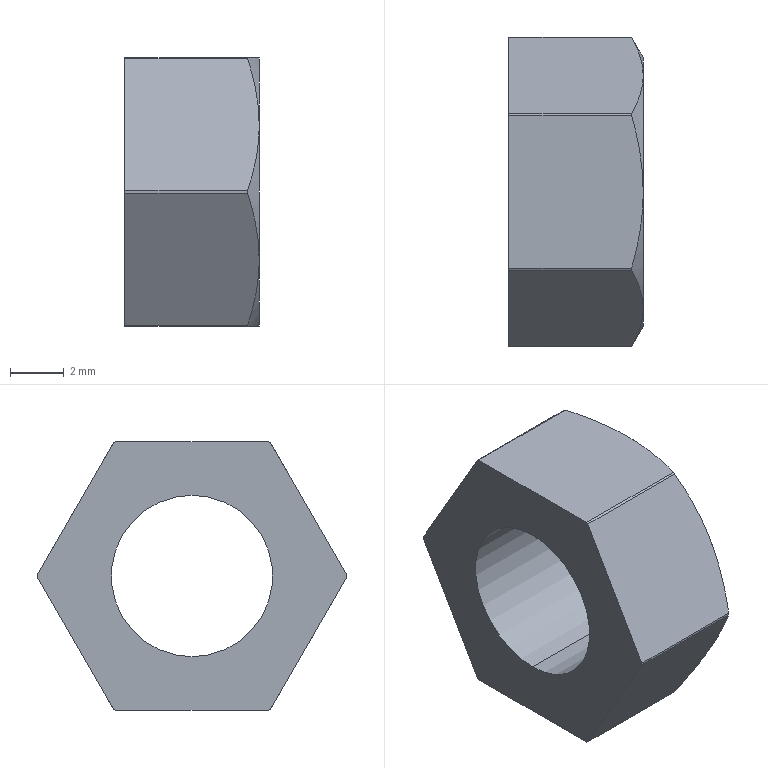Part | STEP file | SSTBB6-25-Part-2-1 | 1 solid | 22 faces | box 5 x 11.5 x 10 mm | volume 290.522 mm3 | cylinder 8 | plane 8 | cone 6 | commonest cylinder face diameters 11.5 x6 6 x2
STEP:
#1=CARTESIAN_POINT('',(12.,0.,3.));
#2=VERTEX_POINT('',#1);
#3=CARTESIAN_POINT('',(12.,0.,-3.));
#4=VERTEX_POINT('',#3);
#5=CARTESIAN_POINT('',(12.,0.,0.));
#6=DIRECTION('',(1.,0.,0.));
#7=DIRECTION('',(0.,0.,1.));
#8=AXIS2_PLACEMENT_3D('',#5,#6,#7);
#9=CIRCLE('',#8,3.);
#10=EDGE_CURVE('',#2,#4,#9,.T.);
#11=ORIENTED_EDGE('',*,*,#10,.T.);
#12=CARTESIAN_POINT('',(7.,0.,-3.));
#13=VERTEX_POINT('',#12);
#14=CARTESIAN_POINT('',(0.,0.,-3.));
#15=DIRECTION('',(-1.,0.,0.));
#16=VECTOR('',#15,1000.);
#17=LINE('',#14,#16);
#18=EDGE_CURVE('',#4,#13,#17,.T.);
#19=ORIENTED_EDGE('',*,*,#18,.T.);
#20=CARTESIAN_POINT('',(7.,0.,3.));
#21=VERTEX_POINT('',#20);
#22=CARTESIAN_POINT('',(7.,0.,0.));
#23=DIRECTION('',(-1.,0.,0.));
#24=DIRECTION('',(0.,0.,-1.));
#25=AXIS2_PLACEMENT_3D('',#22,#23,#24);
#26=CIRCLE('',#25,3.);
#27=EDGE_CURVE('',#13,#21,#26,.T.);
#28=ORIENTED_EDGE('',*,*,#27,.T.);
#29=CARTESIAN_POINT('',(0.,0.,3.));
#30=DIRECTION('',(-1.,0.,0.));
#31=VECTOR('',#30,1000.);
#32=LINE('',#29,#31);
#33=EDGE_CURVE('',#2,#21,#32,.T.);
#34=ORIENTED_EDGE('',*,*,#33,.F.);
#35=EDGE_LOOP('',(#11,#19,#28,#34));
#36=FACE_OUTER_BOUND('',#35,.T.);
#37=CARTESIAN_POINT('',(0.,0.,0.));
#38=DIRECTION('',(-1.,0.,0.));
#39=DIRECTION('',(0.,0.,1.));
#40=AXIS2_PLACEMENT_3D('',#37,#38,#39);
#41=CYLINDRICAL_SURFACE('',#40,3.);
#42=ADVANCED_FACE('',(#36),#41,.F.);
#43=CARTESIAN_POINT('',(11.567,-2.839,-5.));
#44=VERTEX_POINT('',#43);
#45=CARTESIAN_POINT('',(11.567,-2.91,-4.959));
#46=VERTEX_POINT('',#45);
#47=CARTESIAN_POINT('',(11.567,0.,0.));
#48=DIRECTION('',(-1.,0.,0.));
#49=DIRECTION('',(0.,0.,1.));
#50=AXIS2_PLACEMENT_3D('',#47,#48,#49);
#51=CIRCLE('',#50,5.75);
#52=EDGE_CURVE('',#44,#46,#51,.T.);
#53=ORIENTED_EDGE('',*,*,#52,.F.);
#54=CARTESIAN_POINT('',(12.,0.,-5.));
#55=VERTEX_POINT('',#54);
#56=CARTESIAN_POINT('',(11.567,-2.839,-5.));
#57=CARTESIAN_POINT('',(11.831,-1.914,-5.));
#58=CARTESIAN_POINT('',(12.,-0.9721,-5.));
#59=CARTESIAN_POINT('',(12.,0.,-5.));
#60=B_SPLINE_CURVE_WITH_KNOTS('',3,(#56,#57,#58,#59),.UNSPECIFIED.,.F.,.F.,(4,4),(0.006338,0.009225),.UNSPECIFIED.);
#61=EDGE_CURVE('',#44,#55,#60,.T.);
#62=ORIENTED_EDGE('',*,*,#61,.T.);
#63=CARTESIAN_POINT('',(12.,-4.33,-2.5));
#64=VERTEX_POINT('',#63);
#65=CARTESIAN_POINT('',(12.,0.,0.));
#66=DIRECTION('',(-1.,0.,0.));
#67=DIRECTION('',(0.,0.,1.));
#68=AXIS2_PLACEMENT_3D('',#65,#66,#67);
#69=CIRCLE('',#68,5.);
#70=EDGE_CURVE('',#55,#64,#69,.T.);
#71=ORIENTED_EDGE('',*,*,#70,.T.);
#72=CARTESIAN_POINT('',(12.,-4.33,-2.5));
#73=CARTESIAN_POINT('',(12.,-4.21,-2.708));
#74=CARTESIAN_POINT('',(11.99,-4.089,-2.918));
#75=CARTESIAN_POINT('',(11.95,-3.849,-3.333));
#76=CARTESIAN_POINT('',(11.921,-3.73,-3.539));
#77=CARTESIAN_POINT('',(11.808,-3.376,-4.153));
#78=CARTESIAN_POINT('',(11.699,-3.142,-4.558));
#79=CARTESIAN_POINT('',(11.567,-2.91,-4.959));
#80=B_SPLINE_CURVE_WITH_KNOTS('',3,(#72,#73,#74,#75,#76,#77,#78,#79),.UNSPECIFIED.,.F.,.F.,(4,2,2,4),(0.002873,0.003588,0.004303,0.005733),.UNSPECIFIED.);
#81=EDGE_CURVE('',#64,#46,#80,.T.);
#82=ORIENTED_EDGE('',*,*,#81,.T.);
#83=EDGE_LOOP('',(#53,#62,#71,#82));
#84=FACE_OUTER_BOUND('',#83,.T.);
#85=CARTESIAN_POINT('',(12.,0.,0.));
#86=DIRECTION('',(-1.,0.,0.));
#87=DIRECTION('',(0.,0.,1.));
#88=AXIS2_PLACEMENT_3D('',#85,#86,#87);
#89=CONICAL_SURFACE('',#88,5.,1.047);
#90=ADVANCED_FACE('',(#84),#89,.T.);
#91=CARTESIAN_POINT('',(12.,4.33,-2.5));
#92=VERTEX_POINT('',#91);
#93=CARTESIAN_POINT('',(12.,0.,0.));
#94=DIRECTION('',(-1.,0.,0.));
#95=DIRECTION('',(0.,0.,1.));
#96=AXIS2_PLACEMENT_3D('',#93,#94,#95);
#97=CIRCLE('',#96,5.);
#98=EDGE_CURVE('',#92,#55,#97,.T.);
#99=ORIENTED_EDGE('',*,*,#98,.T.);
#100=CARTESIAN_POINT('',(11.567,2.839,-5.));
#101=VERTEX_POINT('',#100);
#102=CARTESIAN_POINT('',(12.,0.,-5.));
#103=CARTESIAN_POINT('',(12.,0.4857,-5.));
#104=CARTESIAN_POINT('',(11.958,0.9657,-5.));
#105=CARTESIAN_POINT('',(11.807,1.911,-5.));
#106=CARTESIAN_POINT('',(11.699,2.377,-5.));
#107=CARTESIAN_POINT('',(11.567,2.839,-5.));
#108=B_SPLINE_CURVE_WITH_KNOTS('',3,(#102,#103,#104,#105,#106,#107),.UNSPECIFIED.,.F.,.F.,(4,2,4),(0.009225,0.01067,0.01211),.UNSPECIFIED.);
#109=EDGE_CURVE('',#55,#101,#108,.T.);
#110=ORIENTED_EDGE('',*,*,#109,.T.);
#111=CARTESIAN_POINT('',(11.567,2.91,-4.959));
#112=VERTEX_POINT('',#111);
#113=CARTESIAN_POINT('',(11.567,0.,0.));
#114=DIRECTION('',(-1.,0.,0.));
#115=DIRECTION('',(0.,0.,1.));
#116=AXIS2_PLACEMENT_3D('',#113,#114,#115);
#117=CIRCLE('',#116,5.75);
#118=EDGE_CURVE('',#112,#101,#117,.T.);
#119=ORIENTED_EDGE('',*,*,#118,.F.);
#120=CARTESIAN_POINT('',(11.567,2.91,-4.959));
#121=CARTESIAN_POINT('',(11.832,3.375,-4.154));
#122=CARTESIAN_POINT('',(12.,3.847,-3.337));
#123=CARTESIAN_POINT('',(12.,4.33,-2.5));
#124=B_SPLINE_CURVE_WITH_KNOTS('',3,(#120,#121,#122,#123),.UNSPECIFIED.,.F.,.F.,(4,4),(0.000000722,0.002873),.UNSPECIFIED.);
#125=EDGE_CURVE('',#112,#92,#124,.T.);
#126=ORIENTED_EDGE('',*,*,#125,.T.);
#127=EDGE_LOOP('',(#99,#110,#119,#126));
#128=FACE_OUTER_BOUND('',#127,.T.);
#129=CARTESIAN_POINT('',(12.,0.,0.));
#130=DIRECTION('',(-1.,0.,0.));
#131=DIRECTION('',(0.,0.,1.));
#132=AXIS2_PLACEMENT_3D('',#129,#130,#131);
#133=CONICAL_SURFACE('',#132,5.,1.047);
#134=ADVANCED_FACE('',(#128),#133,.T.);
#135=CARTESIAN_POINT('',(12.,0.,5.));
#136=VERTEX_POINT('',#135);
#137=CARTESIAN_POINT('',(12.,4.33,2.5));
#138=VERTEX_POINT('',#137);
#139=CARTESIAN_POINT('',(12.,0.,0.));
#140=DIRECTION('',(-1.,0.,0.));
#141=DIRECTION('',(0.,0.,1.));
#142=AXIS2_PLACEMENT_3D('',#139,#140,#141);
#143=CIRCLE('',#142,5.);
#144=EDGE_CURVE('',#136,#138,#143,.T.);
#145=ORIENTED_EDGE('',*,*,#144,.T.);
#146=CARTESIAN_POINT('',(11.567,2.91,4.959));
#147=VERTEX_POINT('',#146);
#148=CARTESIAN_POINT('',(12.,4.33,2.5));
#149=CARTESIAN_POINT('',(12.,4.21,2.708));
#150=CARTESIAN_POINT('',(11.99,4.089,2.918));
#151=CARTESIAN_POINT('',(11.95,3.849,3.333));
#152=CARTESIAN_POINT('',(11.921,3.73,3.539));
#153=CARTESIAN_POINT('',(11.808,3.376,4.153));
#154=CARTESIAN_POINT('',(11.699,3.142,4.558));
#155=CARTESIAN_POINT('',(11.567,2.91,4.959));
#156=B_SPLINE_CURVE_WITH_KNOTS('',3,(#148,#149,#150,#151,#152,#153,#154,#155),.UNSPECIFIED.,.F.,.F.,(4,2,2,4),(0.002873,0.003588,0.004303,0.005733),.UNSPECIFIED.);
#157=EDGE_CURVE('',#138,#147,#156,.T.);
#158=ORIENTED_EDGE('',*,*,#157,.T.);
#159=CARTESIAN_POINT('',(11.567,2.839,5.));
#160=VERTEX_POINT('',#159);
#161=CARTESIAN_POINT('',(11.567,0.,0.));
#162=DIRECTION('',(-1.,0.,0.));
#163=DIRECTION('',(0.,0.,1.));
#164=AXIS2_PLACEMENT_3D('',#161,#162,#163);
#165=CIRCLE('',#164,5.75);
#166=EDGE_CURVE('',#160,#147,#165,.T.);
#167=ORIENTED_EDGE('',*,*,#166,.F.);
#168=CARTESIAN_POINT('',(11.567,2.839,5.));
#169=CARTESIAN_POINT('',(11.831,1.914,5.));
#170=CARTESIAN_POINT('',(12.,0.9721,5.));
#171=CARTESIAN_POINT('',(12.,0.,5.));
#172=B_SPLINE_CURVE_WITH_KNOTS('',3,(#168,#169,#170,#171),.UNSPECIFIED.,.F.,.F.,(4,4),(0.006338,0.009225),.UNSPECIFIED.);
#173=EDGE_CURVE('',#160,#136,#172,.T.);
#174=ORIENTED_EDGE('',*,*,#173,.T.);
#175=EDGE_LOOP('',(#145,#158,#167,#174));
#176=FACE_OUTER_BOUND('',#175,.T.);
#177=CARTESIAN_POINT('',(12.,0.,0.));
#178=DIRECTION('',(-1.,0.,0.));
#179=DIRECTION('',(0.,0.,1.));
#180=AXIS2_PLACEMENT_3D('',#177,#178,#179);
#181=CONICAL_SURFACE('',#180,5.,1.047);
#182=ADVANCED_FACE('',(#176),#181,.T.);
#183=CARTESIAN_POINT('',(12.,-4.33,2.5));
#184=VERTEX_POINT('',#183);
#185=CARTESIAN_POINT('',(12.,0.,0.));
#186=DIRECTION('',(-1.,0.,0.));
#187=DIRECTION('',(0.,0.,1.));
#188=AXIS2_PLACEMENT_3D('',#185,#186,#187);
#189=CIRCLE('',#188,5.);
#190=EDGE_CURVE('',#184,#136,#189,.T.);
#191=ORIENTED_EDGE('',*,*,#190,.T.);
#192=CARTESIAN_POINT('',(11.567,-2.839,5.));
#193=VERTEX_POINT('',#192);
#194=CARTESIAN_POINT('',(12.,0.,5.));
#195=CARTESIAN_POINT('',(12.,-0.4857,5.));
#196=CARTESIAN_POINT('',(11.958,-0.9657,5.));
#197=CARTESIAN_POINT('',(11.807,-1.911,5.));
#198=CARTESIAN_POINT('',(11.699,-2.377,5.));
#199=CARTESIAN_POINT('',(11.567,-2.839,5.));
#200=B_SPLINE_CURVE_WITH_KNOTS('',3,(#194,#195,#196,#197,#198,#199),.UNSPECIFIED.,.F.,.F.,(4,2,4),(0.009225,0.01067,0.01211),.UNSPECIFIED.);
#201=EDGE_CURVE('',#136,#193,#200,.T.);
#202=ORIENTED_EDGE('',*,*,#201,.T.);
#203=CARTESIAN_POINT('',(11.567,-2.91,4.959));
#204=VERTEX_POINT('',#203);
#205=CARTESIAN_POINT('',(11.567,0.,0.));
#206=DIRECTION('',(-1.,0.,0.));
#207=DIRECTION('',(0.,0.,1.));
#208=AXIS2_PLACEMENT_3D('',#205,#206,#207);
#209=CIRCLE('',#208,5.75);
#210=EDGE_CURVE('',#204,#193,#209,.T.);
#211=ORIENTED_EDGE('',*,*,#210,.F.);
#212=CARTESIAN_POINT('',(11.567,-2.91,4.959));
#213=CARTESIAN_POINT('',(11.832,-3.375,4.154));
#214=CARTESIAN_POINT('',(12.,-3.847,3.337));
#215=CARTESIAN_POINT('',(12.,-4.33,2.5));
#216=B_SPLINE_CURVE_WITH_KNOTS('',3,(#212,#213,#214,#215),.UNSPECIFIED.,.F.,.F.,(4,4),(0.000000722,0.002873),.UNSPECIFIED.);
#217=EDGE_CURVE('',#204,#184,#216,.T.);
#218=ORIENTED_EDGE('',*,*,#217,.T.);
#219=EDGE_LOOP('',(#191,#202,#211,#218));
#220=FACE_OUTER_BOUND('',#219,.T.);
#221=CARTESIAN_POINT('',(12.,0.,0.));
#222=DIRECTION('',(-1.,0.,0.));
#223=DIRECTION('',(0.,0.,1.));
#224=AXIS2_PLACEMENT_3D('',#221,#222,#223);
#225=CONICAL_SURFACE('',#224,5.,1.047);
#226=ADVANCED_FACE('',(#220),#225,.T.);
#227=CARTESIAN_POINT('',(12.,0.,0.));
#228=DIRECTION('',(-1.,0.,0.));
#229=DIRECTION('',(0.,0.,1.));
#230=AXIS2_PLACEMENT_3D('',#227,#228,#229);
#231=CIRCLE('',#230,5.);
#232=EDGE_CURVE('',#64,#184,#231,.T.);
#233=ORIENTED_EDGE('',*,*,#232,.T.);
#234=CARTESIAN_POINT('',(11.567,-5.75,0.04096));
#235=VERTEX_POINT('',#234);
#236=CARTESIAN_POINT('',(12.,-4.33,2.5));
#237=CARTESIAN_POINT('',(12.,-4.45,2.292));
#238=CARTESIAN_POINT('',(11.99,-4.571,2.082));
#239=CARTESIAN_POINT('',(11.95,-4.811,1.667));
#240=CARTESIAN_POINT('',(11.921,-4.93,1.461));
#241=CARTESIAN_POINT('',(11.808,-5.284,0.8471));
#242=CARTESIAN_POINT('',(11.699,-5.518,0.4424));
#243=CARTESIAN_POINT('',(11.567,-5.75,0.04096));
#244=B_SPLINE_CURVE_WITH_KNOTS('',3,(#236,#237,#238,#239,#240,#241,#242,#243),.UNSPECIFIED.,.F.,.F.,(4,2,2,4),(0.002873,0.003588,0.004303,0.005733),.UNSPECIFIED.);
#245=EDGE_CURVE('',#184,#235,#244,.T.);
#246=ORIENTED_EDGE('',*,*,#245,.T.);
#247=CARTESIAN_POINT('',(11.567,-5.75,-0.04096));
#248=VERTEX_POINT('',#247);
#249=CARTESIAN_POINT('',(11.567,0.,0.));
#250=DIRECTION('',(-1.,0.,0.));
#251=DIRECTION('',(0.,0.,1.));
#252=AXIS2_PLACEMENT_3D('',#249,#250,#251);
#253=CIRCLE('',#252,5.75);
#254=EDGE_CURVE('',#248,#235,#253,.T.);
#255=ORIENTED_EDGE('',*,*,#254,.F.);
#256=CARTESIAN_POINT('',(11.567,-5.75,-0.04096));
#257=CARTESIAN_POINT('',(11.832,-5.285,-0.8461));
#258=CARTESIAN_POINT('',(12.,-4.813,-1.663));
#259=CARTESIAN_POINT('',(12.,-4.33,-2.5));
#260=B_SPLINE_CURVE_WITH_KNOTS('',3,(#256,#257,#258,#259),.UNSPECIFIED.,.F.,.F.,(4,4),(0.000000712,0.002873),.UNSPECIFIED.);
#261=EDGE_CURVE('',#248,#64,#260,.T.);
#262=ORIENTED_EDGE('',*,*,#261,.T.);
#263=EDGE_LOOP('',(#233,#246,#255,#262));
#264=FACE_OUTER_BOUND('',#263,.T.);
#265=CARTESIAN_POINT('',(12.,0.,0.));
#266=DIRECTION('',(-1.,0.,0.));
#267=DIRECTION('',(0.,0.,1.));
#268=AXIS2_PLACEMENT_3D('',#265,#266,#267);
#269=CONICAL_SURFACE('',#268,5.,1.047);
#270=ADVANCED_FACE('',(#264),#269,.T.);
#271=ORIENTED_EDGE('',*,*,#118,.T.);
#272=CARTESIAN_POINT('',(7.,2.839,-5.));
#273=VERTEX_POINT('',#272);
#274=CARTESIAN_POINT('',(7.,2.839,-5.));
#275=DIRECTION('',(-1.,0.,0.));
#276=VECTOR('',#275,1000.);
#277=LINE('',#274,#276);
#278=EDGE_CURVE('',#101,#273,#277,.T.);
#279=ORIENTED_EDGE('',*,*,#278,.T.);
#280=CARTESIAN_POINT('',(7.,2.91,-4.959));
#281=VERTEX_POINT('',#280);
#282=CARTESIAN_POINT('',(7.,0.,0.));
#283=DIRECTION('',(-1.,0.,0.));
#284=DIRECTION('',(0.,0.,1.));
#285=AXIS2_PLACEMENT_3D('',#282,#283,#284);
#286=CIRCLE('',#285,5.75);
#287=EDGE_CURVE('',#281,#273,#286,.T.);
#288=ORIENTED_EDGE('',*,*,#287,.F.);
#289=CARTESIAN_POINT('',(7.,2.91,-4.959));
#290=DIRECTION('',(1.,0.,0.));
#291=VECTOR('',#290,1000.);
#292=LINE('',#289,#291);
#293=EDGE_CURVE('',#281,#112,#292,.T.);
#294=ORIENTED_EDGE('',*,*,#293,.T.);
#295=EDGE_LOOP('',(#271,#279,#288,#294));
#296=FACE_OUTER_BOUND('',#295,.T.);
#297=CARTESIAN_POINT('',(7.,0.,0.));
#298=DIRECTION('',(-1.,0.,0.));
#299=DIRECTION('',(0.,0.,1.));
#300=AXIS2_PLACEMENT_3D('',#297,#298,#299);
#301=CYLINDRICAL_SURFACE('',#300,5.75);
#302=ADVANCED_FACE('',(#296),#301,.T.);
#303=ORIENTED_EDGE('',*,*,#166,.T.);
#304=CARTESIAN_POINT('',(7.,2.91,4.959));
#305=VERTEX_POINT('',#304);
#306=CARTESIAN_POINT('',(7.,2.91,4.959));
#307=DIRECTION('',(-1.,0.,0.));
#308=VECTOR('',#307,1000.);
#309=LINE('',#306,#308);
#310=EDGE_CURVE('',#147,#305,#309,.T.);
#311=ORIENTED_EDGE('',*,*,#310,.T.);
#312=CARTESIAN_POINT('',(7.,2.839,5.));
#313=VERTEX_POINT('',#312);
#314=CARTESIAN_POINT('',(7.,0.,0.));
#315=DIRECTION('',(-1.,0.,0.));
#316=DIRECTION('',(0.,0.,1.));
#317=AXIS2_PLACEMENT_3D('',#314,#315,#316);
#318=CIRCLE('',#317,5.75);
#319=EDGE_CURVE('',#313,#305,#318,.T.);
#320=ORIENTED_EDGE('',*,*,#319,.F.);
#321=CARTESIAN_POINT('',(7.,2.839,5.));
#322=DIRECTION('',(1.,0.,0.));
#323=VECTOR('',#322,1000.);
#324=LINE('',#321,#323);
#325=EDGE_CURVE('',#313,#160,#324,.T.);
#326=ORIENTED_EDGE('',*,*,#325,.T.);
#327=EDGE_LOOP('',(#303,#311,#320,#326));
#328=FACE_OUTER_BOUND('',#327,.T.);
#329=CARTESIAN_POINT('',(7.,0.,0.));
#330=DIRECTION('',(-1.,0.,0.));
#331=DIRECTION('',(0.,0.,1.));
#332=AXIS2_PLACEMENT_3D('',#329,#330,#331);
#333=CYLINDRICAL_SURFACE('',#332,5.75);
#334=ADVANCED_FACE('',(#328),#333,.T.);
#335=ORIENTED_EDGE('',*,*,#210,.T.);
#336=CARTESIAN_POINT('',(7.,-2.839,5.));
#337=VERTEX_POINT('',#336);
#338=CARTESIAN_POINT('',(7.,-2.839,5.));
#339=DIRECTION('',(-1.,0.,0.));
#340=VECTOR('',#339,1000.);
#341=LINE('',#338,#340);
#342=EDGE_CURVE('',#193,#337,#341,.T.);
#343=ORIENTED_EDGE('',*,*,#342,.T.);
#344=CARTESIAN_POINT('',(7.,-2.91,4.959));
#345=VERTEX_POINT('',#344);
#346=CARTESIAN_POINT('',(7.,0.,0.));
#347=DIRECTION('',(-1.,0.,0.));
#348=DIRECTION('',(0.,0.,1.));
#349=AXIS2_PLACEMENT_3D('',#346,#347,#348);
#350=CIRCLE('',#349,5.75);
#351=EDGE_CURVE('',#345,#337,#350,.T.);
#352=ORIENTED_EDGE('',*,*,#351,.F.);
#353=CARTESIAN_POINT('',(7.,-2.91,4.959));
#354=DIRECTION('',(1.,0.,0.));
#355=VECTOR('',#354,1000.);
#356=LINE('',#353,#355);
#357=EDGE_CURVE('',#345,#204,#356,.T.);
#358=ORIENTED_EDGE('',*,*,#357,.T.);
#359=EDGE_LOOP('',(#335,#343,#352,#358));
#360=FACE_OUTER_BOUND('',#359,.T.);
#361=CARTESIAN_POINT('',(7.,0.,0.));
#362=DIRECTION('',(-1.,0.,0.));
#363=DIRECTION('',(0.,0.,1.));
#364=AXIS2_PLACEMENT_3D('',#361,#362,#363);
#365=CYLINDRICAL_SURFACE('',#364,5.75);
#366=ADVANCED_FACE('',(#360),#365,.T.);
#367=ORIENTED_EDGE('',*,*,#254,.T.);
#368=CARTESIAN_POINT('',(7.,-5.75,0.04096));
#369=VERTEX_POINT('',#368);
#370=CARTESIAN_POINT('',(7.,-5.75,0.04096));
#371=DIRECTION('',(-1.,0.,0.));
#372=VECTOR('',#371,1000.);
#373=LINE('',#370,#372);
#374=EDGE_CURVE('',#235,#369,#373,.T.);
#375=ORIENTED_EDGE('',*,*,#374,.T.);
#376=CARTESIAN_POINT('',(7.,-5.75,-0.04096));
#377=VERTEX_POINT('',#376);
#378=CARTESIAN_POINT('',(7.,0.,0.));
#379=DIRECTION('',(-1.,0.,0.));
#380=DIRECTION('',(0.,0.,1.));
#381=AXIS2_PLACEMENT_3D('',#378,#379,#380);
#382=CIRCLE('',#381,5.75);
#383=EDGE_CURVE('',#377,#369,#382,.T.);
#384=ORIENTED_EDGE('',*,*,#383,.F.);
#385=CARTESIAN_POINT('',(7.,-5.75,-0.04096));
#386=DIRECTION('',(1.,0.,0.));
#387=VECTOR('',#386,1000.);
#388=LINE('',#385,#387);
#389=EDGE_CURVE('',#377,#248,#388,.T.);
#390=ORIENTED_EDGE('',*,*,#389,.T.);
#391=EDGE_LOOP('',(#367,#375,#384,#390));
#392=FACE_OUTER_BOUND('',#391,.T.);
#393=CARTESIAN_POINT('',(7.,0.,0.));
#394=DIRECTION('',(-1.,0.,0.));
#395=DIRECTION('',(0.,0.,1.));
#396=AXIS2_PLACEMENT_3D('',#393,#394,#395);
#397=CYLINDRICAL_SURFACE('',#396,5.75);
#398=ADVANCED_FACE('',(#392),#397,.T.);
#399=CARTESIAN_POINT('',(7.,-2.839,-5.));
#400=VERTEX_POINT('',#399);
#401=CARTESIAN_POINT('',(7.,-2.91,-4.959));
#402=VERTEX_POINT('',#401);
#403=CARTESIAN_POINT('',(7.,0.,0.));
#404=DIRECTION('',(-1.,0.,0.));
#405=DIRECTION('',(0.,0.,1.));
#406=AXIS2_PLACEMENT_3D('',#403,#404,#405);
#407=CIRCLE('',#406,5.75);
#408=EDGE_CURVE('',#400,#402,#407,.T.);
#409=ORIENTED_EDGE('',*,*,#408,.F.);
#410=CARTESIAN_POINT('',(7.,-2.839,-5.));
#411=DIRECTION('',(1.,0.,0.));
#412=VECTOR('',#411,1000.);
#413=LINE('',#410,#412);
#414=EDGE_CURVE('',#400,#44,#413,.T.);
#415=ORIENTED_EDGE('',*,*,#414,.T.);
#416=ORIENTED_EDGE('',*,*,#52,.T.);
#417=CARTESIAN_POINT('',(7.,-2.91,-4.959));
#418=DIRECTION('',(-1.,0.,0.));
#419=VECTOR('',#418,1000.);
#420=LINE('',#417,#419);
#421=EDGE_CURVE('',#46,#402,#420,.T.);
#422=ORIENTED_EDGE('',*,*,#421,.T.);
#423=EDGE_LOOP('',(#409,#415,#416,#422));
#424=FACE_OUTER_BOUND('',#423,.T.);
#425=CARTESIAN_POINT('',(7.,0.,0.));
#426=DIRECTION('',(-1.,0.,0.));
#427=DIRECTION('',(0.,0.,1.));
#428=AXIS2_PLACEMENT_3D('',#425,#426,#427);
#429=CYLINDRICAL_SURFACE('',#428,5.75);
#430=ADVANCED_FACE('',(#424),#429,.T.);
#431=CARTESIAN_POINT('',(12.,0.,0.));
#432=DIRECTION('',(-1.,0.,0.));
#433=DIRECTION('',(0.,0.,1.));
#434=AXIS2_PLACEMENT_3D('',#431,#432,#433);
#435=CIRCLE('',#434,5.);
#436=EDGE_CURVE('',#138,#92,#435,.T.);
#437=ORIENTED_EDGE('',*,*,#436,.F.);
#438=ORIENTED_EDGE('',*,*,#144,.F.);
#439=ORIENTED_EDGE('',*,*,#190,.F.);
#440=ORIENTED_EDGE('',*,*,#232,.F.);
#441=ORIENTED_EDGE('',*,*,#70,.F.);
#442=ORIENTED_EDGE('',*,*,#98,.F.);
#443=EDGE_LOOP('',(#437,#438,#439,#440,#441,#442));
#444=FACE_OUTER_BOUND('',#443,.T.);
#445=ORIENTED_EDGE('',*,*,#10,.F.);
#446=CARTESIAN_POINT('',(12.,0.,0.));
#447=DIRECTION('',(1.,0.,0.));
#448=DIRECTION('',(0.,0.,1.));
#449=AXIS2_PLACEMENT_3D('',#446,#447,#448);
#450=CIRCLE('',#449,3.);
#451=EDGE_CURVE('',#4,#2,#450,.T.);
#452=ORIENTED_EDGE('',*,*,#451,.F.);
#453=EDGE_LOOP('',(#445,#452));
#454=FACE_BOUND('',#453,.T.);
#455=CARTESIAN_POINT('',(12.,0.,0.));
#456=DIRECTION('',(-1.,0.,0.));
#457=DIRECTION('',(0.,0.,1.));
#458=AXIS2_PLACEMENT_3D('',#455,#456,#457);
#459=PLANE('',#458);
#460=ADVANCED_FACE('',(#444,#454),#459,.F.);
#461=ORIENTED_EDGE('',*,*,#436,.T.);
#462=CARTESIAN_POINT('',(11.567,5.75,-0.04096));
#463=VERTEX_POINT('',#462);
#464=CARTESIAN_POINT('',(12.,4.33,-2.5));
#465=CARTESIAN_POINT('',(12.,4.45,-2.292));
#466=CARTESIAN_POINT('',(11.99,4.571,-2.082));
#467=CARTESIAN_POINT('',(11.95,4.811,-1.667));
#468=CARTESIAN_POINT('',(11.921,4.93,-1.461));
#469=CARTESIAN_POINT('',(11.808,5.284,-0.8471));
#470=CARTESIAN_POINT('',(11.699,5.518,-0.4424));
#471=CARTESIAN_POINT('',(11.567,5.75,-0.04096));
#472=B_SPLINE_CURVE_WITH_KNOTS('',3,(#464,#465,#466,#467,#468,#469,#470,#471),.UNSPECIFIED.,.F.,.F.,(4,2,2,4),(0.002873,0.003588,0.004303,0.005733),.UNSPECIFIED.);
#473=EDGE_CURVE('',#92,#463,#472,.T.);
#474=ORIENTED_EDGE('',*,*,#473,.T.);
#475=CARTESIAN_POINT('',(11.567,5.75,0.04096));
#476=VERTEX_POINT('',#475);
#477=CARTESIAN_POINT('',(11.567,0.,0.));
#478=DIRECTION('',(-1.,0.,0.));
#479=DIRECTION('',(0.,0.,1.));
#480=AXIS2_PLACEMENT_3D('',#477,#478,#479);
#481=CIRCLE('',#480,5.75);
#482=EDGE_CURVE('',#476,#463,#481,.T.);
#483=ORIENTED_EDGE('',*,*,#482,.F.);
#484=CARTESIAN_POINT('',(11.567,5.75,0.04096));
#485=CARTESIAN_POINT('',(11.832,5.285,0.8461));
#486=CARTESIAN_POINT('',(12.,4.813,1.663));
#487=CARTESIAN_POINT('',(12.,4.33,2.5));
#488=B_SPLINE_CURVE_WITH_KNOTS('',3,(#484,#485,#486,#487),.UNSPECIFIED.,.F.,.F.,(4,4),(0.000000712,0.002873),.UNSPECIFIED.);
#489=EDGE_CURVE('',#476,#138,#488,.T.);
#490=ORIENTED_EDGE('',*,*,#489,.T.);
#491=EDGE_LOOP('',(#461,#474,#483,#490));
#492=FACE_OUTER_BOUND('',#491,.T.);
#493=CARTESIAN_POINT('',(12.,0.,0.));
#494=DIRECTION('',(-1.,0.,0.));
#495=DIRECTION('',(0.,0.,1.));
#496=AXIS2_PLACEMENT_3D('',#493,#494,#495);
#497=CONICAL_SURFACE('',#496,5.,1.047);
#498=ADVANCED_FACE('',(#492),#497,.T.);
#499=CARTESIAN_POINT('',(7.,5.75,0.04096));
#500=VERTEX_POINT('',#499);
#501=CARTESIAN_POINT('',(7.,5.75,-0.04096));
#502=VERTEX_POINT('',#501);
#503=CARTESIAN_POINT('',(7.,0.,0.));
#504=DIRECTION('',(-1.,0.,0.));
#505=DIRECTION('',(0.,0.,1.));
#506=AXIS2_PLACEMENT_3D('',#503,#504,#505);
#507=CIRCLE('',#506,5.75);
#508=EDGE_CURVE('',#500,#502,#507,.T.);
#509=ORIENTED_EDGE('',*,*,#508,.F.);
#510=CARTESIAN_POINT('',(7.,5.75,0.04096));
#511=DIRECTION('',(1.,0.,0.));
#512=VECTOR('',#511,1000.);
#513=LINE('',#510,#512);
#514=EDGE_CURVE('',#500,#476,#513,.T.);
#515=ORIENTED_EDGE('',*,*,#514,.T.);
#516=ORIENTED_EDGE('',*,*,#482,.T.);
#517=CARTESIAN_POINT('',(7.,5.75,-0.04096));
#518=DIRECTION('',(-1.,0.,0.));
#519=VECTOR('',#518,1000.);
#520=LINE('',#517,#519);
#521=EDGE_CURVE('',#463,#502,#520,.T.);
#522=ORIENTED_EDGE('',*,*,#521,.T.);
#523=EDGE_LOOP('',(#509,#515,#516,#522));
#524=FACE_OUTER_BOUND('',#523,.T.);
#525=CARTESIAN_POINT('',(7.,0.,0.));
#526=DIRECTION('',(-1.,0.,0.));
#527=DIRECTION('',(0.,0.,1.));
#528=AXIS2_PLACEMENT_3D('',#525,#526,#527);
#529=CYLINDRICAL_SURFACE('',#528,5.75);
#530=ADVANCED_FACE('',(#524),#529,.T.);
#531=CARTESIAN_POINT('',(7.,0.,0.));
#532=DIRECTION('',(-1.,0.,0.));
#533=DIRECTION('',(0.,0.,-1.));
#534=AXIS2_PLACEMENT_3D('',#531,#532,#533);
#535=CIRCLE('',#534,3.);
#536=EDGE_CURVE('',#21,#13,#535,.T.);
#537=ORIENTED_EDGE('',*,*,#536,.F.);
#538=ORIENTED_EDGE('',*,*,#27,.F.);
#539=EDGE_LOOP('',(#537,#538));
#540=FACE_BOUND('',#539,.T.);
#541=CARTESIAN_POINT('',(7.,5.768,0.01018));
#542=DIRECTION('',(0.,0.5,-0.866));
#543=VECTOR('',#542,1000.);
#544=LINE('',#541,#543);
#545=EDGE_CURVE('',#305,#500,#544,.T.);
#546=ORIENTED_EDGE('',*,*,#545,.T.);
#547=ORIENTED_EDGE('',*,*,#508,.T.);
#548=CARTESIAN_POINT('',(7.,5.768,-0.01018));
#549=DIRECTION('',(0.,-0.5,-0.866));
#550=VECTOR('',#549,1000.);
#551=LINE('',#548,#550);
#552=EDGE_CURVE('',#502,#281,#551,.T.);
#553=ORIENTED_EDGE('',*,*,#552,.T.);
#554=ORIENTED_EDGE('',*,*,#287,.T.);
#555=CARTESIAN_POINT('',(7.,5.75,-5.));
#556=DIRECTION('',(0.,-1.,0.));
#557=VECTOR('',#556,1000.);
#558=LINE('',#555,#557);
#559=EDGE_CURVE('',#273,#400,#558,.T.);
#560=ORIENTED_EDGE('',*,*,#559,.T.);
#561=ORIENTED_EDGE('',*,*,#408,.T.);
#562=CARTESIAN_POINT('',(7.,-2.893,-4.99));
#563=DIRECTION('',(0.,-0.5,0.866));
#564=VECTOR('',#563,1000.);
#565=LINE('',#562,#564);
#566=EDGE_CURVE('',#402,#377,#565,.T.);
#567=ORIENTED_EDGE('',*,*,#566,.T.);
#568=ORIENTED_EDGE('',*,*,#383,.T.);
#569=CARTESIAN_POINT('',(7.,-2.893,4.99));
#570=DIRECTION('',(0.,0.5,0.866));
#571=VECTOR('',#570,1000.);
#572=LINE('',#569,#571);
#573=EDGE_CURVE('',#369,#345,#572,.T.);
#574=ORIENTED_EDGE('',*,*,#573,.T.);
#575=ORIENTED_EDGE('',*,*,#351,.T.);
#576=CARTESIAN_POINT('',(7.,5.75,5.));
#577=DIRECTION('',(0.,1.,0.));
#578=VECTOR('',#577,1000.);
#579=LINE('',#576,#578);
#580=EDGE_CURVE('',#337,#313,#579,.T.);
#581=ORIENTED_EDGE('',*,*,#580,.T.);
#582=ORIENTED_EDGE('',*,*,#319,.T.);
#583=EDGE_LOOP('',(#546,#547,#553,#554,#560,#561,#567,#568,#574,#575,#581,#582));
#584=FACE_OUTER_BOUND('',#583,.T.);
#585=CARTESIAN_POINT('',(7.,5.75,0.));
#586=DIRECTION('',(1.,0.,0.));
#587=DIRECTION('',(0.,0.,-1.));
#588=AXIS2_PLACEMENT_3D('',#585,#586,#587);
#589=PLANE('',#588);
#590=ADVANCED_FACE('',(#540,#584),#589,.F.);
#591=ORIENTED_EDGE('',*,*,#81,.F.);
#592=ORIENTED_EDGE('',*,*,#261,.F.);
#593=ORIENTED_EDGE('',*,*,#389,.F.);
#594=ORIENTED_EDGE('',*,*,#566,.F.);
#595=ORIENTED_EDGE('',*,*,#421,.F.);
#596=EDGE_LOOP('',(#591,#592,#593,#594,#595));
#597=FACE_OUTER_BOUND('',#596,.T.);
#598=CARTESIAN_POINT('',(7.,-2.887,-5.));
#599=DIRECTION('',(0.,0.866,0.5));
#600=DIRECTION('',(0.,0.5,-0.866));
#601=AXIS2_PLACEMENT_3D('',#598,#599,#600);
#602=PLANE('',#601);
#603=ADVANCED_FACE('',(#597),#602,.F.);
#604=ORIENTED_EDGE('',*,*,#245,.F.);
#605=ORIENTED_EDGE('',*,*,#217,.F.);
#606=ORIENTED_EDGE('',*,*,#357,.F.);
#607=ORIENTED_EDGE('',*,*,#573,.F.);
#608=ORIENTED_EDGE('',*,*,#374,.F.);
#609=EDGE_LOOP('',(#604,#605,#606,#607,#608));
#610=FACE_OUTER_BOUND('',#609,.T.);
#611=CARTESIAN_POINT('',(7.,-5.774,0.));
#612=DIRECTION('',(0.,0.866,-0.5));
#613=DIRECTION('',(0.,-0.5,-0.866));
#614=AXIS2_PLACEMENT_3D('',#611,#612,#613);
#615=PLANE('',#614);
#616=ADVANCED_FACE('',(#610),#615,.F.);
#617=ORIENTED_EDGE('',*,*,#201,.F.);
#618=ORIENTED_EDGE('',*,*,#173,.F.);
#619=ORIENTED_EDGE('',*,*,#325,.F.);
#620=ORIENTED_EDGE('',*,*,#580,.F.);
#621=ORIENTED_EDGE('',*,*,#342,.F.);
#622=EDGE_LOOP('',(#617,#618,#619,#620,#621));
#623=FACE_OUTER_BOUND('',#622,.T.);
#624=CARTESIAN_POINT('',(7.,-2.887,5.));
#625=DIRECTION('',(0.,0.,-1.));
#626=DIRECTION('',(-1.,0.,0.));
#627=AXIS2_PLACEMENT_3D('',#624,#625,#626);
#628=PLANE('',#627);
#629=ADVANCED_FACE('',(#623),#628,.F.);
#630=ORIENTED_EDGE('',*,*,#157,.F.);
#631=ORIENTED_EDGE('',*,*,#489,.F.);
#632=ORIENTED_EDGE('',*,*,#514,.F.);
#633=ORIENTED_EDGE('',*,*,#545,.F.);
#634=ORIENTED_EDGE('',*,*,#310,.F.);
#635=EDGE_LOOP('',(#630,#631,#632,#633,#634));
#636=FACE_OUTER_BOUND('',#635,.T.);
#637=CARTESIAN_POINT('',(7.,2.887,5.));
#638=DIRECTION('',(0.,-0.866,-0.5));
#639=DIRECTION('',(0.,-0.5,0.866));
#640=AXIS2_PLACEMENT_3D('',#637,#638,#639);
#641=PLANE('',#640);
#642=ADVANCED_FACE('',(#636),#641,.F.);
#643=ORIENTED_EDGE('',*,*,#473,.F.);
#644=ORIENTED_EDGE('',*,*,#125,.F.);
#645=ORIENTED_EDGE('',*,*,#293,.F.);
#646=ORIENTED_EDGE('',*,*,#552,.F.);
#647=ORIENTED_EDGE('',*,*,#521,.F.);
#648=EDGE_LOOP('',(#643,#644,#645,#646,#647));
#649=FACE_OUTER_BOUND('',#648,.T.);
#650=CARTESIAN_POINT('',(7.,5.774,0.));
#651=DIRECTION('',(0.,-0.866,0.5));
#652=DIRECTION('',(0.,0.5,0.866));
#653=AXIS2_PLACEMENT_3D('',#650,#651,#652);
#654=PLANE('',#653);
#655=ADVANCED_FACE('',(#649),#654,.F.);
#656=ORIENTED_EDGE('',*,*,#109,.F.);
#657=ORIENTED_EDGE('',*,*,#61,.F.);
#658=ORIENTED_EDGE('',*,*,#414,.F.);
#659=ORIENTED_EDGE('',*,*,#559,.F.);
#660=ORIENTED_EDGE('',*,*,#278,.F.);
#661=EDGE_LOOP('',(#656,#657,#658,#659,#660));
#662=FACE_OUTER_BOUND('',#661,.T.);
#663=CARTESIAN_POINT('',(7.,2.887,-5.));
#664=DIRECTION('',(0.,0.,1.));
#665=DIRECTION('',(1.,0.,0.));
#666=AXIS2_PLACEMENT_3D('',#663,#664,#665);
#667=PLANE('',#666);
#668=ADVANCED_FACE('',(#662),#667,.F.);
#669=ORIENTED_EDGE('',*,*,#18,.F.);
#670=ORIENTED_EDGE('',*,*,#451,.T.);
#671=ORIENTED_EDGE('',*,*,#33,.T.);
#672=ORIENTED_EDGE('',*,*,#536,.T.);
#673=EDGE_LOOP('',(#669,#670,#671,#672));
#674=FACE_OUTER_BOUND('',#673,.T.);
#675=CARTESIAN_POINT('',(0.,0.,0.));
#676=DIRECTION('',(-1.,0.,0.));
#677=DIRECTION('',(0.,0.,1.));
#678=AXIS2_PLACEMENT_3D('',#675,#676,#677);
#679=CYLINDRICAL_SURFACE('',#678,3.);
#680=ADVANCED_FACE('',(#674),#679,.F.);
#681=CLOSED_SHELL('',(#42,#90,#134,#182,#226,#270,#302,#334,#366,#398,#430,#460,#498,#530,#590,#603,#616,#629,#642,#655,#668,#680));
#682=MANIFOLD_SOLID_BREP('',#681);
#683=CARTESIAN_POINT('',(0.,0.,0.));
#684=DIRECTION('',(0.,0.,1.));
#685=DIRECTION('',(1.,0.,0.));
#686=AXIS2_PLACEMENT_3D('',#683,#684,#685);
#687=(LENGTH_UNIT()NAMED_UNIT(*)SI_UNIT(.MILLI.,.METRE.));
#688=UNCERTAINTY_MEASURE_WITH_UNIT(LENGTH_MEASURE(0.00001),#687,'','');
#689=(NAMED_UNIT(*)PLANE_ANGLE_UNIT()SI_UNIT($,.RADIAN.));
#690=(NAMED_UNIT(*)SI_UNIT($,.STERADIAN.)SOLID_ANGLE_UNIT());
#691=(GEOMETRIC_REPRESENTATION_CONTEXT(3)GLOBAL_UNCERTAINTY_ASSIGNED_CONTEXT((#688))GLOBAL_UNIT_ASSIGNED_CONTEXT((#687,#689,#690))REPRESENTATION_CONTEXT('',''));
#692=ADVANCED_BREP_SHAPE_REPRESENTATION('',(#682,#686),#691);